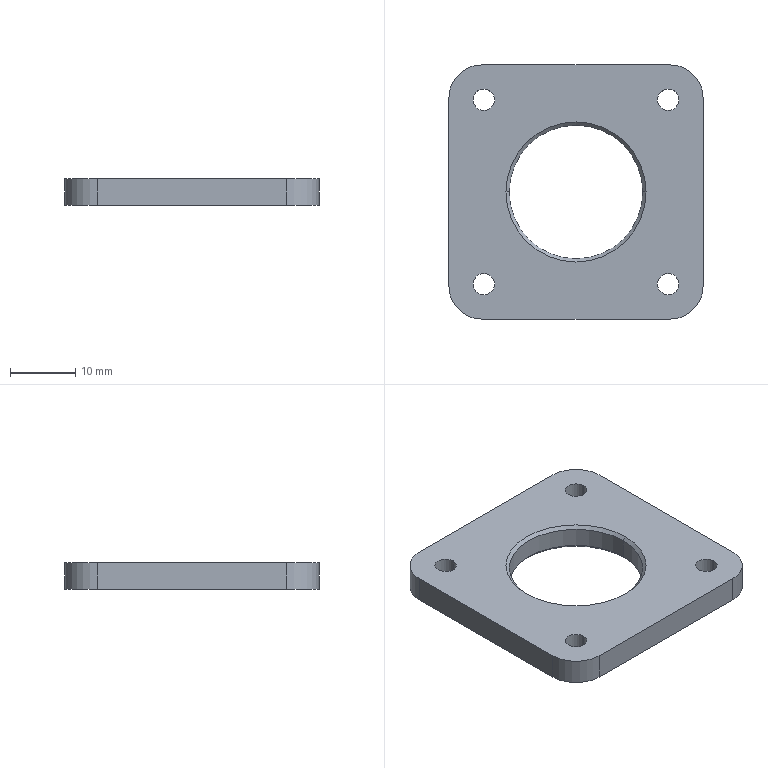Part | NX | features BREP 1 | 1 solid | 24 faces | box 39 x 39 x 4 mm | volume 4525 mm3 | cylinder 14 | plane 6 | cone 4 | commonest cylinder face diameters 3.3 x8 10 x4 20.5 x2
STEP:
#1=CARTESIAN_POINT('',(-10.75,0.,4.));
#2=VERTEX_POINT('',#1);
#3=CARTESIAN_POINT('',(-10.25,0.,3.5));
#4=VERTEX_POINT('',#3);
#5=CARTESIAN_POINT('',(-10.25,0.,3.5));
#6=DIRECTION('',(-0.7071,0.,0.7071));
#7=VECTOR('',#6,1000.);
#8=LINE('',#5,#7);
#9=EDGE_CURVE('',#2,#4,#8,.F.);
#10=ORIENTED_EDGE('',*,*,#9,.T.);
#11=CARTESIAN_POINT('',(10.25,0.,3.5));
#12=VERTEX_POINT('',#11);
#13=CARTESIAN_POINT('',(0.,0.,3.5));
#14=DIRECTION('',(0.,0.,1.));
#15=DIRECTION('',(-1.,0.,0.));
#16=AXIS2_PLACEMENT_3D('',#13,#14,#15);
#17=CIRCLE('',#16,10.25);
#18=EDGE_CURVE('',#12,#4,#17,.T.);
#19=ORIENTED_EDGE('',*,*,#18,.F.);
#20=CARTESIAN_POINT('',(10.75,0.,4.));
#21=VERTEX_POINT('',#20);
#22=CARTESIAN_POINT('',(10.25,0.,3.5));
#23=DIRECTION('',(0.7071,0.,0.7071));
#24=VECTOR('',#23,1000.);
#25=LINE('',#22,#24);
#26=EDGE_CURVE('',#21,#12,#25,.F.);
#27=ORIENTED_EDGE('',*,*,#26,.F.);
#28=CARTESIAN_POINT('',(0.,0.,4.));
#29=DIRECTION('',(0.,0.,-1.));
#30=DIRECTION('',(-1.,0.,0.));
#31=AXIS2_PLACEMENT_3D('',#28,#29,#30);
#32=CIRCLE('',#31,10.75);
#33=EDGE_CURVE('',#2,#21,#32,.T.);
#34=ORIENTED_EDGE('',*,*,#33,.F.);
#35=EDGE_LOOP('',(#10,#19,#27,#34));
#36=FACE_BOUND('',#35,.T.);
#37=CARTESIAN_POINT('',(0.,0.,3.5));
#38=DIRECTION('',(0.,0.,1.));
#39=DIRECTION('',(1.,0.,0.));
#40=AXIS2_PLACEMENT_3D('',#37,#38,#39);
#41=CONICAL_SURFACE('',#40,10.25,0.7854);
#42=ADVANCED_FACE('',(#36),#41,.F.);
#43=CARTESIAN_POINT('',(10.25,0.,0.5));
#44=VERTEX_POINT('',#43);
#45=CARTESIAN_POINT('',(10.75,0.,0.));
#46=VERTEX_POINT('',#45);
#47=CARTESIAN_POINT('',(10.75,0.,0.));
#48=DIRECTION('',(0.7071,0.,-0.7071));
#49=VECTOR('',#48,1000.);
#50=LINE('',#47,#49);
#51=EDGE_CURVE('',#44,#46,#50,.T.);
#52=ORIENTED_EDGE('',*,*,#51,.F.);
#53=CARTESIAN_POINT('',(-10.25,0.,0.5));
#54=VERTEX_POINT('',#53);
#55=CARTESIAN_POINT('',(0.,0.,0.5));
#56=DIRECTION('',(0.,0.,-1.));
#57=DIRECTION('',(-1.,0.,0.));
#58=AXIS2_PLACEMENT_3D('',#55,#56,#57);
#59=CIRCLE('',#58,10.25);
#60=EDGE_CURVE('',#54,#44,#59,.T.);
#61=ORIENTED_EDGE('',*,*,#60,.F.);
#62=CARTESIAN_POINT('',(-10.75,0.,0.));
#63=VERTEX_POINT('',#62);
#64=CARTESIAN_POINT('',(-10.75,0.,0.));
#65=DIRECTION('',(-0.7071,0.,-0.7071));
#66=VECTOR('',#65,1000.);
#67=LINE('',#64,#66);
#68=EDGE_CURVE('',#54,#63,#67,.T.);
#69=ORIENTED_EDGE('',*,*,#68,.T.);
#70=CARTESIAN_POINT('',(0.,0.,0.));
#71=DIRECTION('',(0.,0.,1.));
#72=DIRECTION('',(-1.,0.,0.));
#73=AXIS2_PLACEMENT_3D('',#70,#71,#72);
#74=CIRCLE('',#73,10.75);
#75=EDGE_CURVE('',#46,#63,#74,.T.);
#76=ORIENTED_EDGE('',*,*,#75,.F.);
#77=EDGE_LOOP('',(#52,#61,#69,#76));
#78=FACE_BOUND('',#77,.T.);
#79=CARTESIAN_POINT('',(0.,0.,0.));
#80=DIRECTION('',(0.,0.,-1.));
#81=DIRECTION('',(-1.,0.,0.));
#82=AXIS2_PLACEMENT_3D('',#79,#80,#81);
#83=CONICAL_SURFACE('',#82,10.75,0.7854);
#84=ADVANCED_FACE('',(#78),#83,.F.);
#85=CARTESIAN_POINT('',(12.492,14.142,4.));
#86=VERTEX_POINT('',#85);
#87=CARTESIAN_POINT('',(12.492,14.142,0.));
#88=VERTEX_POINT('',#87);
#89=CARTESIAN_POINT('',(12.492,14.142,4.));
#90=DIRECTION('',(0.,0.,1.));
#91=VECTOR('',#90,1000.);
#92=LINE('',#89,#91);
#93=EDGE_CURVE('',#86,#88,#92,.F.);
#94=ORIENTED_EDGE('',*,*,#93,.T.);
#95=CARTESIAN_POINT('',(15.792,14.142,0.));
#96=VERTEX_POINT('',#95);
#97=CARTESIAN_POINT('',(14.142,14.142,0.));
#98=DIRECTION('',(0.,0.,-1.));
#99=DIRECTION('',(-1.,0.,0.));
#100=AXIS2_PLACEMENT_3D('',#97,#98,#99);
#101=CIRCLE('',#100,1.65);
#102=EDGE_CURVE('',#88,#96,#101,.T.);
#103=ORIENTED_EDGE('',*,*,#102,.T.);
#104=CARTESIAN_POINT('',(15.792,14.142,4.));
#105=VERTEX_POINT('',#104);
#106=CARTESIAN_POINT('',(15.792,14.142,4.));
#107=DIRECTION('',(0.,0.,1.));
#108=VECTOR('',#107,1000.);
#109=LINE('',#106,#108);
#110=EDGE_CURVE('',#105,#96,#109,.F.);
#111=ORIENTED_EDGE('',*,*,#110,.F.);
#112=CARTESIAN_POINT('',(14.142,14.142,4.));
#113=DIRECTION('',(0.,0.,1.));
#114=DIRECTION('',(1.,0.,0.));
#115=AXIS2_PLACEMENT_3D('',#112,#113,#114);
#116=CIRCLE('',#115,1.65);
#117=EDGE_CURVE('',#105,#86,#116,.T.);
#118=ORIENTED_EDGE('',*,*,#117,.T.);
#119=EDGE_LOOP('',(#94,#103,#111,#118));
#120=FACE_BOUND('',#119,.T.);
#121=CARTESIAN_POINT('',(14.142,14.142,4.));
#122=DIRECTION('',(0.,0.,1.));
#123=DIRECTION('',(1.,0.,0.));
#124=AXIS2_PLACEMENT_3D('',#121,#122,#123);
#125=CYLINDRICAL_SURFACE('',#124,1.65);
#126=ADVANCED_FACE('',(#120),#125,.F.);
#127=CARTESIAN_POINT('',(12.492,-14.142,4.));
#128=VERTEX_POINT('',#127);
#129=CARTESIAN_POINT('',(12.492,-14.142,0.));
#130=VERTEX_POINT('',#129);
#131=CARTESIAN_POINT('',(12.492,-14.142,4.));
#132=DIRECTION('',(0.,0.,1.));
#133=VECTOR('',#132,1000.);
#134=LINE('',#131,#133);
#135=EDGE_CURVE('',#128,#130,#134,.F.);
#136=ORIENTED_EDGE('',*,*,#135,.T.);
#137=CARTESIAN_POINT('',(15.792,-14.142,0.));
#138=VERTEX_POINT('',#137);
#139=CARTESIAN_POINT('',(14.142,-14.142,0.));
#140=DIRECTION('',(0.,0.,-1.));
#141=DIRECTION('',(-1.,0.,0.));
#142=AXIS2_PLACEMENT_3D('',#139,#140,#141);
#143=CIRCLE('',#142,1.65);
#144=EDGE_CURVE('',#130,#138,#143,.T.);
#145=ORIENTED_EDGE('',*,*,#144,.T.);
#146=CARTESIAN_POINT('',(15.792,-14.142,4.));
#147=VERTEX_POINT('',#146);
#148=CARTESIAN_POINT('',(15.792,-14.142,4.));
#149=DIRECTION('',(0.,0.,1.));
#150=VECTOR('',#149,1000.);
#151=LINE('',#148,#150);
#152=EDGE_CURVE('',#147,#138,#151,.F.);
#153=ORIENTED_EDGE('',*,*,#152,.F.);
#154=CARTESIAN_POINT('',(14.142,-14.142,4.));
#155=DIRECTION('',(0.,0.,1.));
#156=DIRECTION('',(1.,0.,0.));
#157=AXIS2_PLACEMENT_3D('',#154,#155,#156);
#158=CIRCLE('',#157,1.65);
#159=EDGE_CURVE('',#147,#128,#158,.T.);
#160=ORIENTED_EDGE('',*,*,#159,.T.);
#161=EDGE_LOOP('',(#136,#145,#153,#160));
#162=FACE_BOUND('',#161,.T.);
#163=CARTESIAN_POINT('',(14.142,-14.142,4.));
#164=DIRECTION('',(0.,0.,1.));
#165=DIRECTION('',(1.,0.,0.));
#166=AXIS2_PLACEMENT_3D('',#163,#164,#165);
#167=CYLINDRICAL_SURFACE('',#166,1.65);
#168=ADVANCED_FACE('',(#162),#167,.F.);
#169=CARTESIAN_POINT('',(-15.792,-14.142,4.));
#170=VERTEX_POINT('',#169);
#171=CARTESIAN_POINT('',(-15.792,-14.142,0.));
#172=VERTEX_POINT('',#171);
#173=CARTESIAN_POINT('',(-15.792,-14.142,4.));
#174=DIRECTION('',(0.,0.,1.));
#175=VECTOR('',#174,1000.);
#176=LINE('',#173,#175);
#177=EDGE_CURVE('',#170,#172,#176,.F.);
#178=ORIENTED_EDGE('',*,*,#177,.T.);
#179=CARTESIAN_POINT('',(-12.492,-14.142,0.));
#180=VERTEX_POINT('',#179);
#181=CARTESIAN_POINT('',(-14.142,-14.142,0.));
#182=DIRECTION('',(0.,0.,-1.));
#183=DIRECTION('',(-1.,0.,0.));
#184=AXIS2_PLACEMENT_3D('',#181,#182,#183);
#185=CIRCLE('',#184,1.65);
#186=EDGE_CURVE('',#172,#180,#185,.T.);
#187=ORIENTED_EDGE('',*,*,#186,.T.);
#188=CARTESIAN_POINT('',(-12.492,-14.142,4.));
#189=VERTEX_POINT('',#188);
#190=CARTESIAN_POINT('',(-12.492,-14.142,4.));
#191=DIRECTION('',(0.,0.,1.));
#192=VECTOR('',#191,1000.);
#193=LINE('',#190,#192);
#194=EDGE_CURVE('',#189,#180,#193,.F.);
#195=ORIENTED_EDGE('',*,*,#194,.F.);
#196=CARTESIAN_POINT('',(-14.142,-14.142,4.));
#197=DIRECTION('',(0.,0.,1.));
#198=DIRECTION('',(1.,0.,0.));
#199=AXIS2_PLACEMENT_3D('',#196,#197,#198);
#200=CIRCLE('',#199,1.65);
#201=EDGE_CURVE('',#189,#170,#200,.T.);
#202=ORIENTED_EDGE('',*,*,#201,.T.);
#203=EDGE_LOOP('',(#178,#187,#195,#202));
#204=FACE_BOUND('',#203,.T.);
#205=CARTESIAN_POINT('',(-14.142,-14.142,4.));
#206=DIRECTION('',(0.,0.,1.));
#207=DIRECTION('',(1.,0.,0.));
#208=AXIS2_PLACEMENT_3D('',#205,#206,#207);
#209=CYLINDRICAL_SURFACE('',#208,1.65);
#210=ADVANCED_FACE('',(#204),#209,.F.);
#211=CARTESIAN_POINT('',(-15.792,14.142,4.));
#212=VERTEX_POINT('',#211);
#213=CARTESIAN_POINT('',(-15.792,14.142,0.));
#214=VERTEX_POINT('',#213);
#215=CARTESIAN_POINT('',(-15.792,14.142,4.));
#216=DIRECTION('',(0.,0.,1.));
#217=VECTOR('',#216,1000.);
#218=LINE('',#215,#217);
#219=EDGE_CURVE('',#212,#214,#218,.F.);
#220=ORIENTED_EDGE('',*,*,#219,.T.);
#221=CARTESIAN_POINT('',(-12.492,14.142,0.));
#222=VERTEX_POINT('',#221);
#223=CARTESIAN_POINT('',(-14.142,14.142,0.));
#224=DIRECTION('',(0.,0.,-1.));
#225=DIRECTION('',(-1.,0.,0.));
#226=AXIS2_PLACEMENT_3D('',#223,#224,#225);
#227=CIRCLE('',#226,1.65);
#228=EDGE_CURVE('',#214,#222,#227,.T.);
#229=ORIENTED_EDGE('',*,*,#228,.T.);
#230=CARTESIAN_POINT('',(-12.492,14.142,4.));
#231=VERTEX_POINT('',#230);
#232=CARTESIAN_POINT('',(-12.492,14.142,4.));
#233=DIRECTION('',(0.,0.,1.));
#234=VECTOR('',#233,1000.);
#235=LINE('',#232,#234);
#236=EDGE_CURVE('',#231,#222,#235,.F.);
#237=ORIENTED_EDGE('',*,*,#236,.F.);
#238=CARTESIAN_POINT('',(-14.142,14.142,4.));
#239=DIRECTION('',(0.,0.,1.));
#240=DIRECTION('',(1.,0.,0.));
#241=AXIS2_PLACEMENT_3D('',#238,#239,#240);
#242=CIRCLE('',#241,1.65);
#243=EDGE_CURVE('',#231,#212,#242,.T.);
#244=ORIENTED_EDGE('',*,*,#243,.T.);
#245=EDGE_LOOP('',(#220,#229,#237,#244));
#246=FACE_BOUND('',#245,.T.);
#247=CARTESIAN_POINT('',(-14.142,14.142,4.));
#248=DIRECTION('',(0.,0.,1.));
#249=DIRECTION('',(1.,0.,0.));
#250=AXIS2_PLACEMENT_3D('',#247,#248,#249);
#251=CYLINDRICAL_SURFACE('',#250,1.65);
#252=ADVANCED_FACE('',(#246),#251,.F.);
#253=CARTESIAN_POINT('',(19.5,14.5,4.));
#254=VERTEX_POINT('',#253);
#255=CARTESIAN_POINT('',(14.5,19.5,4.));
#256=VERTEX_POINT('',#255);
#257=CARTESIAN_POINT('',(14.5,14.5,4.));
#258=DIRECTION('',(0.,0.,1.));
#259=DIRECTION('',(-1.,0.,0.));
#260=AXIS2_PLACEMENT_3D('',#257,#258,#259);
#261=CIRCLE('',#260,5.);
#262=EDGE_CURVE('',#254,#256,#261,.T.);
#263=ORIENTED_EDGE('',*,*,#262,.F.);
#264=CARTESIAN_POINT('',(19.5,14.5,0.));
#265=VERTEX_POINT('',#264);
#266=CARTESIAN_POINT('',(19.5,14.5,4.));
#267=DIRECTION('',(0.,0.,1.));
#268=VECTOR('',#267,1000.);
#269=LINE('',#266,#268);
#270=EDGE_CURVE('',#265,#254,#269,.T.);
#271=ORIENTED_EDGE('',*,*,#270,.F.);
#272=CARTESIAN_POINT('',(14.5,19.5,0.));
#273=VERTEX_POINT('',#272);
#274=CARTESIAN_POINT('',(14.5,14.5,0.));
#275=DIRECTION('',(0.,0.,-1.));
#276=DIRECTION('',(-1.,0.,0.));
#277=AXIS2_PLACEMENT_3D('',#274,#275,#276);
#278=CIRCLE('',#277,5.);
#279=EDGE_CURVE('',#273,#265,#278,.T.);
#280=ORIENTED_EDGE('',*,*,#279,.F.);
#281=CARTESIAN_POINT('',(14.5,19.5,4.));
#282=DIRECTION('',(0.,0.,-1.));
#283=VECTOR('',#282,1000.);
#284=LINE('',#281,#283);
#285=EDGE_CURVE('',#256,#273,#284,.T.);
#286=ORIENTED_EDGE('',*,*,#285,.F.);
#287=EDGE_LOOP('',(#263,#271,#280,#286));
#288=FACE_BOUND('',#287,.T.);
#289=CARTESIAN_POINT('',(14.5,14.5,4.));
#290=DIRECTION('',(0.,0.,-1.));
#291=DIRECTION('',(-1.,0.,0.));
#292=AXIS2_PLACEMENT_3D('',#289,#290,#291);
#293=CYLINDRICAL_SURFACE('',#292,5.);
#294=ADVANCED_FACE('',(#288),#293,.T.);
#295=CARTESIAN_POINT('',(-14.5,19.5,4.));
#296=VERTEX_POINT('',#295);
#297=CARTESIAN_POINT('',(-19.5,14.5,4.));
#298=VERTEX_POINT('',#297);
#299=CARTESIAN_POINT('',(-14.5,14.5,4.));
#300=DIRECTION('',(0.,0.,1.));
#301=DIRECTION('',(-1.,0.,0.));
#302=AXIS2_PLACEMENT_3D('',#299,#300,#301);
#303=CIRCLE('',#302,5.);
#304=EDGE_CURVE('',#296,#298,#303,.T.);
#305=ORIENTED_EDGE('',*,*,#304,.F.);
#306=CARTESIAN_POINT('',(-14.5,19.5,0.));
#307=VERTEX_POINT('',#306);
#308=CARTESIAN_POINT('',(-14.5,19.5,4.));
#309=DIRECTION('',(0.,0.,1.));
#310=VECTOR('',#309,1000.);
#311=LINE('',#308,#310);
#312=EDGE_CURVE('',#307,#296,#311,.T.);
#313=ORIENTED_EDGE('',*,*,#312,.F.);
#314=CARTESIAN_POINT('',(-19.5,14.5,0.));
#315=VERTEX_POINT('',#314);
#316=CARTESIAN_POINT('',(-14.5,14.5,0.));
#317=DIRECTION('',(0.,0.,-1.));
#318=DIRECTION('',(-1.,0.,0.));
#319=AXIS2_PLACEMENT_3D('',#316,#317,#318);
#320=CIRCLE('',#319,5.);
#321=EDGE_CURVE('',#315,#307,#320,.T.);
#322=ORIENTED_EDGE('',*,*,#321,.F.);
#323=CARTESIAN_POINT('',(-19.5,14.5,4.));
#324=DIRECTION('',(0.,0.,-1.));
#325=VECTOR('',#324,1000.);
#326=LINE('',#323,#325);
#327=EDGE_CURVE('',#298,#315,#326,.T.);
#328=ORIENTED_EDGE('',*,*,#327,.F.);
#329=EDGE_LOOP('',(#305,#313,#322,#328));
#330=FACE_BOUND('',#329,.T.);
#331=CARTESIAN_POINT('',(-14.5,14.5,4.));
#332=DIRECTION('',(0.,0.,-1.));
#333=DIRECTION('',(-1.,0.,0.));
#334=AXIS2_PLACEMENT_3D('',#331,#332,#333);
#335=CYLINDRICAL_SURFACE('',#334,5.);
#336=ADVANCED_FACE('',(#330),#335,.T.);
#337=CARTESIAN_POINT('',(14.5,-19.5,4.));
#338=VERTEX_POINT('',#337);
#339=CARTESIAN_POINT('',(19.5,-14.5,4.));
#340=VERTEX_POINT('',#339);
#341=CARTESIAN_POINT('',(14.5,-14.5,4.));
#342=DIRECTION('',(0.,0.,1.));
#343=DIRECTION('',(-1.,0.,0.));
#344=AXIS2_PLACEMENT_3D('',#341,#342,#343);
#345=CIRCLE('',#344,5.);
#346=EDGE_CURVE('',#338,#340,#345,.T.);
#347=ORIENTED_EDGE('',*,*,#346,.F.);
#348=CARTESIAN_POINT('',(14.5,-19.5,0.));
#349=VERTEX_POINT('',#348);
#350=CARTESIAN_POINT('',(14.5,-19.5,4.));
#351=DIRECTION('',(0.,0.,1.));
#352=VECTOR('',#351,1000.);
#353=LINE('',#350,#352);
#354=EDGE_CURVE('',#349,#338,#353,.T.);
#355=ORIENTED_EDGE('',*,*,#354,.F.);
#356=CARTESIAN_POINT('',(19.5,-14.5,0.));
#357=VERTEX_POINT('',#356);
#358=CARTESIAN_POINT('',(14.5,-14.5,0.));
#359=DIRECTION('',(0.,0.,-1.));
#360=DIRECTION('',(-1.,0.,0.));
#361=AXIS2_PLACEMENT_3D('',#358,#359,#360);
#362=CIRCLE('',#361,5.);
#363=EDGE_CURVE('',#357,#349,#362,.T.);
#364=ORIENTED_EDGE('',*,*,#363,.F.);
#365=CARTESIAN_POINT('',(19.5,-14.5,4.));
#366=DIRECTION('',(0.,0.,-1.));
#367=VECTOR('',#366,1000.);
#368=LINE('',#365,#367);
#369=EDGE_CURVE('',#340,#357,#368,.T.);
#370=ORIENTED_EDGE('',*,*,#369,.F.);
#371=EDGE_LOOP('',(#347,#355,#364,#370));
#372=FACE_BOUND('',#371,.T.);
#373=CARTESIAN_POINT('',(14.5,-14.5,4.));
#374=DIRECTION('',(0.,0.,-1.));
#375=DIRECTION('',(-1.,0.,0.));
#376=AXIS2_PLACEMENT_3D('',#373,#374,#375);
#377=CYLINDRICAL_SURFACE('',#376,5.);
#378=ADVANCED_FACE('',(#372),#377,.T.);
#379=CARTESIAN_POINT('',(-19.5,-14.5,4.));
#380=VERTEX_POINT('',#379);
#381=CARTESIAN_POINT('',(-14.5,-19.5,4.));
#382=VERTEX_POINT('',#381);
#383=CARTESIAN_POINT('',(-14.5,-14.5,4.));
#384=DIRECTION('',(0.,0.,1.));
#385=DIRECTION('',(-1.,0.,0.));
#386=AXIS2_PLACEMENT_3D('',#383,#384,#385);
#387=CIRCLE('',#386,5.);
#388=EDGE_CURVE('',#380,#382,#387,.T.);
#389=ORIENTED_EDGE('',*,*,#388,.F.);
#390=CARTESIAN_POINT('',(-19.5,-14.5,0.));
#391=VERTEX_POINT('',#390);
#392=CARTESIAN_POINT('',(-19.5,-14.5,4.));
#393=DIRECTION('',(0.,0.,1.));
#394=VECTOR('',#393,1000.);
#395=LINE('',#392,#394);
#396=EDGE_CURVE('',#391,#380,#395,.T.);
#397=ORIENTED_EDGE('',*,*,#396,.F.);
#398=CARTESIAN_POINT('',(-14.5,-19.5,0.));
#399=VERTEX_POINT('',#398);
#400=CARTESIAN_POINT('',(-14.5,-14.5,0.));
#401=DIRECTION('',(0.,0.,-1.));
#402=DIRECTION('',(-1.,0.,0.));
#403=AXIS2_PLACEMENT_3D('',#400,#401,#402);
#404=CIRCLE('',#403,5.);
#405=EDGE_CURVE('',#399,#391,#404,.T.);
#406=ORIENTED_EDGE('',*,*,#405,.F.);
#407=CARTESIAN_POINT('',(-14.5,-19.5,4.));
#408=DIRECTION('',(0.,0.,-1.));
#409=VECTOR('',#408,1000.);
#410=LINE('',#407,#409);
#411=EDGE_CURVE('',#382,#399,#410,.T.);
#412=ORIENTED_EDGE('',*,*,#411,.F.);
#413=EDGE_LOOP('',(#389,#397,#406,#412));
#414=FACE_BOUND('',#413,.T.);
#415=CARTESIAN_POINT('',(-14.5,-14.5,4.));
#416=DIRECTION('',(0.,0.,-1.));
#417=DIRECTION('',(-1.,0.,0.));
#418=AXIS2_PLACEMENT_3D('',#415,#416,#417);
#419=CYLINDRICAL_SURFACE('',#418,5.);
#420=ADVANCED_FACE('',(#414),#419,.T.);
#421=CARTESIAN_POINT('',(10.25,0.,4.));
#422=DIRECTION('',(0.,0.,-1.));
#423=VECTOR('',#422,1000.);
#424=LINE('',#421,#423);
#425=EDGE_CURVE('',#12,#44,#424,.T.);
#426=ORIENTED_EDGE('',*,*,#425,.F.);
#427=ORIENTED_EDGE('',*,*,#18,.T.);
#428=CARTESIAN_POINT('',(-10.25,0.,4.));
#429=DIRECTION('',(0.,0.,-1.));
#430=VECTOR('',#429,1000.);
#431=LINE('',#428,#430);
#432=EDGE_CURVE('',#4,#54,#431,.T.);
#433=ORIENTED_EDGE('',*,*,#432,.T.);
#434=ORIENTED_EDGE('',*,*,#60,.T.);
#435=EDGE_LOOP('',(#426,#427,#433,#434));
#436=FACE_BOUND('',#435,.T.);
#437=CARTESIAN_POINT('',(0.,0.,4.));
#438=DIRECTION('',(0.,0.,-1.));
#439=DIRECTION('',(-1.,0.,0.));
#440=AXIS2_PLACEMENT_3D('',#437,#438,#439);
#441=CYLINDRICAL_SURFACE('',#440,10.25);
#442=ADVANCED_FACE('',(#436),#441,.F.);
#443=CARTESIAN_POINT('',(19.5,19.5,0.));
#444=DIRECTION('',(-1.,0.,0.));
#445=VECTOR('',#444,1000.);
#446=LINE('',#443,#445);
#447=EDGE_CURVE('',#273,#307,#446,.T.);
#448=ORIENTED_EDGE('',*,*,#447,.T.);
#449=ORIENTED_EDGE('',*,*,#312,.T.);
#450=CARTESIAN_POINT('',(19.5,19.5,4.));
#451=DIRECTION('',(-1.,0.,0.));
#452=VECTOR('',#451,1000.);
#453=LINE('',#450,#452);
#454=EDGE_CURVE('',#256,#296,#453,.T.);
#455=ORIENTED_EDGE('',*,*,#454,.F.);
#456=ORIENTED_EDGE('',*,*,#285,.T.);
#457=EDGE_LOOP('',(#448,#449,#455,#456));
#458=FACE_BOUND('',#457,.T.);
#459=CARTESIAN_POINT('',(19.5,19.5,4.));
#460=DIRECTION('',(0.,-1.,0.));
#461=DIRECTION('',(1.,0.,0.));
#462=AXIS2_PLACEMENT_3D('',#459,#460,#461);
#463=PLANE('',#462);
#464=ADVANCED_FACE('',(#458),#463,.F.);
#465=CARTESIAN_POINT('',(19.5,19.5,4.));
#466=DIRECTION('',(0.,1.,0.));
#467=VECTOR('',#466,1000.);
#468=LINE('',#465,#467);
#469=EDGE_CURVE('',#340,#254,#468,.T.);
#470=ORIENTED_EDGE('',*,*,#469,.F.);
#471=ORIENTED_EDGE('',*,*,#369,.T.);
#472=CARTESIAN_POINT('',(19.5,19.5,0.));
#473=DIRECTION('',(0.,1.,0.));
#474=VECTOR('',#473,1000.);
#475=LINE('',#472,#474);
#476=EDGE_CURVE('',#357,#265,#475,.T.);
#477=ORIENTED_EDGE('',*,*,#476,.T.);
#478=ORIENTED_EDGE('',*,*,#270,.T.);
#479=EDGE_LOOP('',(#470,#471,#477,#478));
#480=FACE_BOUND('',#479,.T.);
#481=CARTESIAN_POINT('',(19.5,19.5,4.));
#482=DIRECTION('',(-1.,0.,0.));
#483=DIRECTION('',(0.,-1.,0.));
#484=AXIS2_PLACEMENT_3D('',#481,#482,#483);
#485=PLANE('',#484);
#486=ADVANCED_FACE('',(#480),#485,.F.);
#487=CARTESIAN_POINT('',(19.5,-19.5,4.));
#488=DIRECTION('',(1.,0.,0.));
#489=VECTOR('',#488,1000.);
#490=LINE('',#487,#489);
#491=EDGE_CURVE('',#382,#338,#490,.T.);
#492=ORIENTED_EDGE('',*,*,#491,.F.);
#493=ORIENTED_EDGE('',*,*,#411,.T.);
#494=CARTESIAN_POINT('',(19.5,-19.5,0.));
#495=DIRECTION('',(1.,0.,0.));
#496=VECTOR('',#495,1000.);
#497=LINE('',#494,#496);
#498=EDGE_CURVE('',#399,#349,#497,.T.);
#499=ORIENTED_EDGE('',*,*,#498,.T.);
#500=ORIENTED_EDGE('',*,*,#354,.T.);
#501=EDGE_LOOP('',(#492,#493,#499,#500));
#502=FACE_BOUND('',#501,.T.);
#503=CARTESIAN_POINT('',(19.5,-19.5,4.));
#504=DIRECTION('',(0.,1.,0.));
#505=DIRECTION('',(-1.,0.,0.));
#506=AXIS2_PLACEMENT_3D('',#503,#504,#505);
#507=PLANE('',#506);
#508=ADVANCED_FACE('',(#502),#507,.F.);
#509=CARTESIAN_POINT('',(-19.5,19.5,0.));
#510=DIRECTION('',(0.,-1.,0.));
#511=VECTOR('',#510,1000.);
#512=LINE('',#509,#511);
#513=EDGE_CURVE('',#315,#391,#512,.T.);
#514=ORIENTED_EDGE('',*,*,#513,.T.);
#515=ORIENTED_EDGE('',*,*,#396,.T.);
#516=CARTESIAN_POINT('',(-19.5,19.5,4.));
#517=DIRECTION('',(0.,-1.,0.));
#518=VECTOR('',#517,1000.);
#519=LINE('',#516,#518);
#520=EDGE_CURVE('',#298,#380,#519,.T.);
#521=ORIENTED_EDGE('',*,*,#520,.F.);
#522=ORIENTED_EDGE('',*,*,#327,.T.);
#523=EDGE_LOOP('',(#514,#515,#521,#522));
#524=FACE_BOUND('',#523,.T.);
#525=CARTESIAN_POINT('',(-19.5,19.5,4.));
#526=DIRECTION('',(1.,0.,0.));
#527=DIRECTION('',(0.,1.,0.));
#528=AXIS2_PLACEMENT_3D('',#525,#526,#527);
#529=PLANE('',#528);
#530=ADVANCED_FACE('',(#524),#529,.F.);
#531=ORIENTED_EDGE('',*,*,#498,.F.);
#532=ORIENTED_EDGE('',*,*,#405,.T.);
#533=ORIENTED_EDGE('',*,*,#513,.F.);
#534=ORIENTED_EDGE('',*,*,#321,.T.);
#535=ORIENTED_EDGE('',*,*,#447,.F.);
#536=ORIENTED_EDGE('',*,*,#279,.T.);
#537=ORIENTED_EDGE('',*,*,#476,.F.);
#538=ORIENTED_EDGE('',*,*,#363,.T.);
#539=EDGE_LOOP('',(#531,#532,#533,#534,#535,#536,#537,#538));
#540=FACE_BOUND('',#539,.T.);
#541=CARTESIAN_POINT('',(-14.142,14.142,0.));
#542=DIRECTION('',(0.,0.,-1.));
#543=DIRECTION('',(-1.,0.,0.));
#544=AXIS2_PLACEMENT_3D('',#541,#542,#543);
#545=CIRCLE('',#544,1.65);
#546=EDGE_CURVE('',#222,#214,#545,.T.);
#547=ORIENTED_EDGE('',*,*,#546,.F.);
#548=ORIENTED_EDGE('',*,*,#228,.F.);
#549=EDGE_LOOP('',(#547,#548));
#550=FACE_BOUND('',#549,.T.);
#551=CARTESIAN_POINT('',(-14.142,-14.142,0.));
#552=DIRECTION('',(0.,0.,-1.));
#553=DIRECTION('',(-1.,0.,0.));
#554=AXIS2_PLACEMENT_3D('',#551,#552,#553);
#555=CIRCLE('',#554,1.65);
#556=EDGE_CURVE('',#180,#172,#555,.T.);
#557=ORIENTED_EDGE('',*,*,#556,.F.);
#558=ORIENTED_EDGE('',*,*,#186,.F.);
#559=EDGE_LOOP('',(#557,#558));
#560=FACE_BOUND('',#559,.T.);
#561=CARTESIAN_POINT('',(14.142,-14.142,0.));
#562=DIRECTION('',(0.,0.,-1.));
#563=DIRECTION('',(-1.,0.,0.));
#564=AXIS2_PLACEMENT_3D('',#561,#562,#563);
#565=CIRCLE('',#564,1.65);
#566=EDGE_CURVE('',#138,#130,#565,.T.);
#567=ORIENTED_EDGE('',*,*,#566,.F.);
#568=ORIENTED_EDGE('',*,*,#144,.F.);
#569=EDGE_LOOP('',(#567,#568));
#570=FACE_BOUND('',#569,.T.);
#571=CARTESIAN_POINT('',(14.142,14.142,0.));
#572=DIRECTION('',(0.,0.,-1.));
#573=DIRECTION('',(-1.,0.,0.));
#574=AXIS2_PLACEMENT_3D('',#571,#572,#573);
#575=CIRCLE('',#574,1.65);
#576=EDGE_CURVE('',#96,#88,#575,.T.);
#577=ORIENTED_EDGE('',*,*,#576,.F.);
#578=ORIENTED_EDGE('',*,*,#102,.F.);
#579=EDGE_LOOP('',(#577,#578));
#580=FACE_BOUND('',#579,.T.);
#581=CARTESIAN_POINT('',(0.,0.,0.));
#582=DIRECTION('',(0.,0.,1.));
#583=DIRECTION('',(-1.,0.,0.));
#584=AXIS2_PLACEMENT_3D('',#581,#582,#583);
#585=CIRCLE('',#584,10.75);
#586=EDGE_CURVE('',#63,#46,#585,.T.);
#587=ORIENTED_EDGE('',*,*,#586,.T.);
#588=ORIENTED_EDGE('',*,*,#75,.T.);
#589=EDGE_LOOP('',(#587,#588));
#590=FACE_BOUND('',#589,.T.);
#591=CARTESIAN_POINT('',(0.,0.,0.));
#592=DIRECTION('',(0.,0.,-1.));
#593=DIRECTION('',(-1.,0.,0.));
#594=AXIS2_PLACEMENT_3D('',#591,#592,#593);
#595=PLANE('',#594);
#596=ADVANCED_FACE('',(#540,#550,#560,#570,#580,#590),#595,.T.);
#597=ORIENTED_EDGE('',*,*,#201,.F.);
#598=CARTESIAN_POINT('',(-14.142,-14.142,4.));
#599=DIRECTION('',(0.,0.,1.));
#600=DIRECTION('',(1.,0.,0.));
#601=AXIS2_PLACEMENT_3D('',#598,#599,#600);
#602=CIRCLE('',#601,1.65);
#603=EDGE_CURVE('',#170,#189,#602,.T.);
#604=ORIENTED_EDGE('',*,*,#603,.F.);
#605=EDGE_LOOP('',(#597,#604));
#606=FACE_BOUND('',#605,.T.);
#607=ORIENTED_EDGE('',*,*,#520,.T.);
#608=ORIENTED_EDGE('',*,*,#388,.T.);
#609=ORIENTED_EDGE('',*,*,#491,.T.);
#610=ORIENTED_EDGE('',*,*,#346,.T.);
#611=ORIENTED_EDGE('',*,*,#469,.T.);
#612=ORIENTED_EDGE('',*,*,#262,.T.);
#613=ORIENTED_EDGE('',*,*,#454,.T.);
#614=ORIENTED_EDGE('',*,*,#304,.T.);
#615=EDGE_LOOP('',(#607,#608,#609,#610,#611,#612,#613,#614));
#616=FACE_BOUND('',#615,.T.);
#617=ORIENTED_EDGE('',*,*,#243,.F.);
#618=CARTESIAN_POINT('',(-14.142,14.142,4.));
#619=DIRECTION('',(0.,0.,1.));
#620=DIRECTION('',(1.,0.,0.));
#621=AXIS2_PLACEMENT_3D('',#618,#619,#620);
#622=CIRCLE('',#621,1.65);
#623=EDGE_CURVE('',#212,#231,#622,.T.);
#624=ORIENTED_EDGE('',*,*,#623,.F.);
#625=EDGE_LOOP('',(#617,#624));
#626=FACE_BOUND('',#625,.T.);
#627=ORIENTED_EDGE('',*,*,#159,.F.);
#628=CARTESIAN_POINT('',(14.142,-14.142,4.));
#629=DIRECTION('',(0.,0.,1.));
#630=DIRECTION('',(1.,0.,0.));
#631=AXIS2_PLACEMENT_3D('',#628,#629,#630);
#632=CIRCLE('',#631,1.65);
#633=EDGE_CURVE('',#128,#147,#632,.T.);
#634=ORIENTED_EDGE('',*,*,#633,.F.);
#635=EDGE_LOOP('',(#627,#634));
#636=FACE_BOUND('',#635,.T.);
#637=ORIENTED_EDGE('',*,*,#117,.F.);
#638=CARTESIAN_POINT('',(14.142,14.142,4.));
#639=DIRECTION('',(0.,0.,1.));
#640=DIRECTION('',(1.,0.,0.));
#641=AXIS2_PLACEMENT_3D('',#638,#639,#640);
#642=CIRCLE('',#641,1.65);
#643=EDGE_CURVE('',#86,#105,#642,.T.);
#644=ORIENTED_EDGE('',*,*,#643,.F.);
#645=EDGE_LOOP('',(#637,#644));
#646=FACE_BOUND('',#645,.T.);
#647=CARTESIAN_POINT('',(0.,0.,4.));
#648=DIRECTION('',(0.,0.,-1.));
#649=DIRECTION('',(-1.,0.,0.));
#650=AXIS2_PLACEMENT_3D('',#647,#648,#649);
#651=CIRCLE('',#650,10.75);
#652=EDGE_CURVE('',#21,#2,#651,.T.);
#653=ORIENTED_EDGE('',*,*,#652,.T.);
#654=ORIENTED_EDGE('',*,*,#33,.T.);
#655=EDGE_LOOP('',(#653,#654));
#656=FACE_BOUND('',#655,.T.);
#657=CARTESIAN_POINT('',(0.,0.,4.));
#658=DIRECTION('',(0.,0.,-1.));
#659=DIRECTION('',(-1.,0.,0.));
#660=AXIS2_PLACEMENT_3D('',#657,#658,#659);
#661=PLANE('',#660);
#662=ADVANCED_FACE('',(#606,#616,#626,#636,#646,#656),#661,.F.);
#663=CARTESIAN_POINT('',(0.,0.,3.5));
#664=DIRECTION('',(0.,0.,1.));
#665=DIRECTION('',(-1.,0.,0.));
#666=AXIS2_PLACEMENT_3D('',#663,#664,#665);
#667=CIRCLE('',#666,10.25);
#668=EDGE_CURVE('',#4,#12,#667,.T.);
#669=ORIENTED_EDGE('',*,*,#668,.T.);
#670=ORIENTED_EDGE('',*,*,#425,.T.);
#671=CARTESIAN_POINT('',(0.,0.,0.5));
#672=DIRECTION('',(0.,0.,-1.));
#673=DIRECTION('',(-1.,0.,0.));
#674=AXIS2_PLACEMENT_3D('',#671,#672,#673);
#675=CIRCLE('',#674,10.25);
#676=EDGE_CURVE('',#44,#54,#675,.T.);
#677=ORIENTED_EDGE('',*,*,#676,.T.);
#678=ORIENTED_EDGE('',*,*,#432,.F.);
#679=EDGE_LOOP('',(#669,#670,#677,#678));
#680=FACE_BOUND('',#679,.T.);
#681=CARTESIAN_POINT('',(0.,0.,4.));
#682=DIRECTION('',(0.,0.,-1.));
#683=DIRECTION('',(-1.,0.,0.));
#684=AXIS2_PLACEMENT_3D('',#681,#682,#683);
#685=CYLINDRICAL_SURFACE('',#684,10.25);
#686=ADVANCED_FACE('',(#680),#685,.F.);
#687=ORIENTED_EDGE('',*,*,#546,.T.);
#688=ORIENTED_EDGE('',*,*,#219,.F.);
#689=ORIENTED_EDGE('',*,*,#623,.T.);
#690=ORIENTED_EDGE('',*,*,#236,.T.);
#691=EDGE_LOOP('',(#687,#688,#689,#690));
#692=FACE_BOUND('',#691,.T.);
#693=CARTESIAN_POINT('',(-14.142,14.142,4.));
#694=DIRECTION('',(0.,0.,1.));
#695=DIRECTION('',(1.,0.,0.));
#696=AXIS2_PLACEMENT_3D('',#693,#694,#695);
#697=CYLINDRICAL_SURFACE('',#696,1.65);
#698=ADVANCED_FACE('',(#692),#697,.F.);
#699=ORIENTED_EDGE('',*,*,#556,.T.);
#700=ORIENTED_EDGE('',*,*,#177,.F.);
#701=ORIENTED_EDGE('',*,*,#603,.T.);
#702=ORIENTED_EDGE('',*,*,#194,.T.);
#703=EDGE_LOOP('',(#699,#700,#701,#702));
#704=FACE_BOUND('',#703,.T.);
#705=CARTESIAN_POINT('',(-14.142,-14.142,4.));
#706=DIRECTION('',(0.,0.,1.));
#707=DIRECTION('',(1.,0.,0.));
#708=AXIS2_PLACEMENT_3D('',#705,#706,#707);
#709=CYLINDRICAL_SURFACE('',#708,1.65);
#710=ADVANCED_FACE('',(#704),#709,.F.);
#711=ORIENTED_EDGE('',*,*,#566,.T.);
#712=ORIENTED_EDGE('',*,*,#135,.F.);
#713=ORIENTED_EDGE('',*,*,#633,.T.);
#714=ORIENTED_EDGE('',*,*,#152,.T.);
#715=EDGE_LOOP('',(#711,#712,#713,#714));
#716=FACE_BOUND('',#715,.T.);
#717=CARTESIAN_POINT('',(14.142,-14.142,4.));
#718=DIRECTION('',(0.,0.,1.));
#719=DIRECTION('',(1.,0.,0.));
#720=AXIS2_PLACEMENT_3D('',#717,#718,#719);
#721=CYLINDRICAL_SURFACE('',#720,1.65);
#722=ADVANCED_FACE('',(#716),#721,.F.);
#723=ORIENTED_EDGE('',*,*,#576,.T.);
#724=ORIENTED_EDGE('',*,*,#93,.F.);
#725=ORIENTED_EDGE('',*,*,#643,.T.);
#726=ORIENTED_EDGE('',*,*,#110,.T.);
#727=EDGE_LOOP('',(#723,#724,#725,#726));
#728=FACE_BOUND('',#727,.T.);
#729=CARTESIAN_POINT('',(14.142,14.142,4.));
#730=DIRECTION('',(0.,0.,1.));
#731=DIRECTION('',(1.,0.,0.));
#732=AXIS2_PLACEMENT_3D('',#729,#730,#731);
#733=CYLINDRICAL_SURFACE('',#732,1.65);
#734=ADVANCED_FACE('',(#728),#733,.F.);
#735=ORIENTED_EDGE('',*,*,#676,.F.);
#736=ORIENTED_EDGE('',*,*,#51,.T.);
#737=ORIENTED_EDGE('',*,*,#586,.F.);
#738=ORIENTED_EDGE('',*,*,#68,.F.);
#739=EDGE_LOOP('',(#735,#736,#737,#738));
#740=FACE_BOUND('',#739,.T.);
#741=CARTESIAN_POINT('',(0.,0.,0.));
#742=DIRECTION('',(0.,0.,-1.));
#743=DIRECTION('',(-1.,0.,0.));
#744=AXIS2_PLACEMENT_3D('',#741,#742,#743);
#745=CONICAL_SURFACE('',#744,10.75,0.7854);
#746=ADVANCED_FACE('',(#740),#745,.F.);
#747=ORIENTED_EDGE('',*,*,#668,.F.);
#748=ORIENTED_EDGE('',*,*,#9,.F.);
#749=ORIENTED_EDGE('',*,*,#652,.F.);
#750=ORIENTED_EDGE('',*,*,#26,.T.);
#751=EDGE_LOOP('',(#747,#748,#749,#750));
#752=FACE_BOUND('',#751,.T.);
#753=CARTESIAN_POINT('',(0.,0.,3.5));
#754=DIRECTION('',(0.,0.,1.));
#755=DIRECTION('',(1.,0.,0.));
#756=AXIS2_PLACEMENT_3D('',#753,#754,#755);
#757=CONICAL_SURFACE('',#756,10.25,0.7854);
#758=ADVANCED_FACE('',(#752),#757,.F.);
#759=CLOSED_SHELL('',(#42,#84,#126,#168,#210,#252,#294,#336,#378,#420,#442,#464,#486,#508,#530,#596,#662,#686,#698,#710,#722,#734,#746,#758));
#760=MANIFOLD_SOLID_BREP('',#759);
#761=(LENGTH_UNIT()NAMED_UNIT(*)SI_UNIT(.MILLI.,.METRE.));
#762=UNCERTAINTY_MEASURE_WITH_UNIT(LENGTH_MEASURE(0.00001),#761,'','');
#763=(NAMED_UNIT(*)PLANE_ANGLE_UNIT()SI_UNIT($,.RADIAN.));
#764=(NAMED_UNIT(*)SI_UNIT($,.STERADIAN.)SOLID_ANGLE_UNIT());
#765=(GEOMETRIC_REPRESENTATION_CONTEXT(3)GLOBAL_UNCERTAINTY_ASSIGNED_CONTEXT((#762))GLOBAL_UNIT_ASSIGNED_CONTEXT((#761,#763,#764))REPRESENTATION_CONTEXT('',''));
#766=ADVANCED_BREP_SHAPE_REPRESENTATION('',(#760),#765);